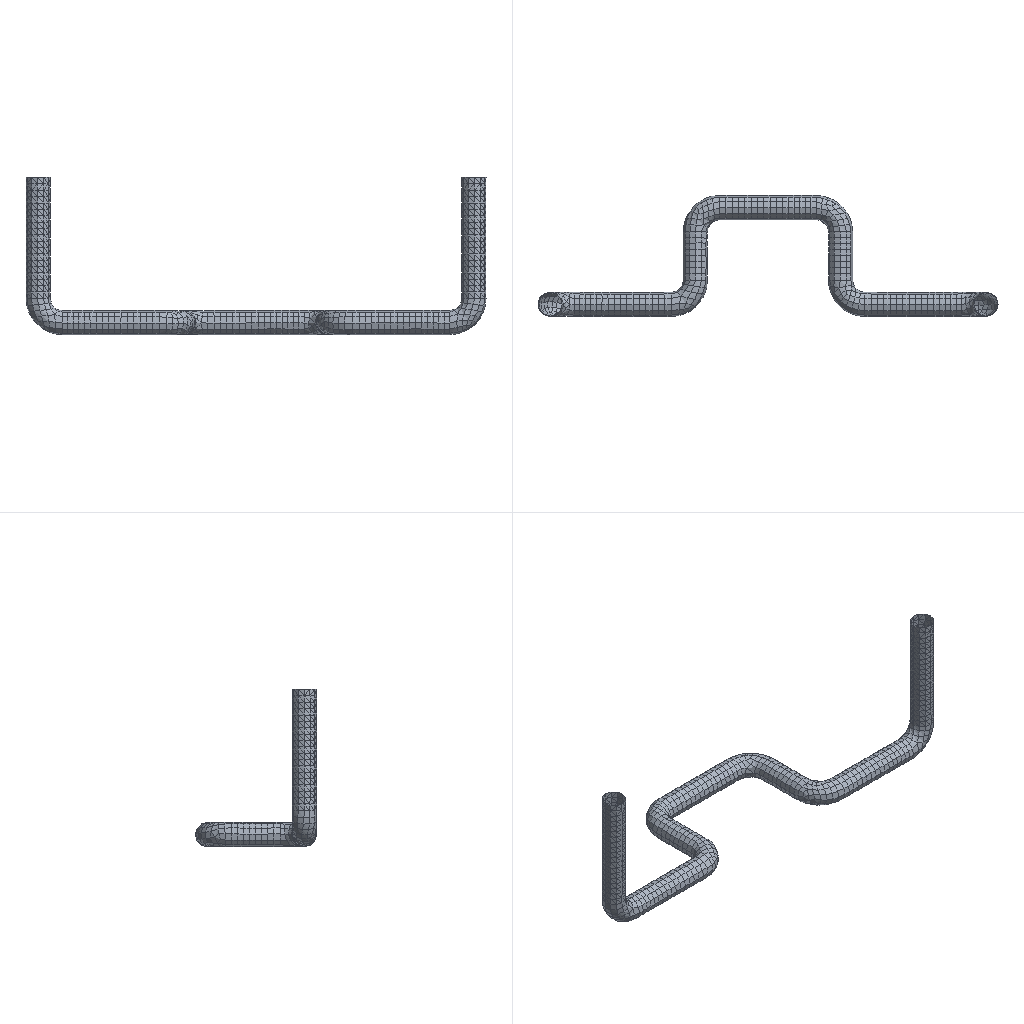Simulation study | ansys workbench
Set-up summary:
category,name,step,type,value,unit,region
solver,ansys_workbench
units,mm-N-s-tonne (MPa),,stated,"/units,MPA"
analysis,LS1,,transient
load_step,LS1,LS1,transient,time=1
mesh,nodes,,,1720
mesh,elements,,,3874
element_type,SHELL181,,,1709
element_type,SURF154,,,1709
element_type,CONTA174,,,456
material,Structural Steel,,E,200000,tonne s^-2 mm^-1
material,Structural Steel,,nu,0.3
material,Structural Steel,,density,7.85e-09,tonne mm^-3
material,Structural Steel,,conductivity,60.5,tonne mm s^-3 C^-1
material,Structural Steel,,specific_heat,4.34e+08,mm^2 s^-2 C^-1
material,Structural Steel,,cte,1.2e-05,C^-1
material,Structural Steel,,permeability,10000
material,Structural Steel,,resistivity,0.00017,ohm mm
load,ACEL,LS1,gravity (ACEL; gravity acts opposite),"9806.65 [dir=(0, -1, 0)]",,all
load,"Create Imported Load ""Imported Pressure""",LS1,pressure,1.094 [n=1709],,element list
bc,Constant Zero Displacement X,model,fixed,[dofs=UX],,_DISPZEROUX
bc,Constant Zero Displacement Z,model,fixed,[dofs=UZ],,_DISPZEROUZ
bc,"Create Spring Connection ""Longitudinal - Ground To Surface Body""",model,fixed,[dofs=ALL n=2],,node list
contact,contact 1,,bonded (always),element=CONTA174
contact,contact 2,,bonded (always),element=CONTA174
named_set,WALL,,node,1716
named_set,_DISPZEROUX,,node,1716
named_set,_DISPZEROUZ,,node,1716
named_set,ALLGROUNDEDSPRINGS,,node,2
Ansys APDL input file, long lists of numbers shortened:
/batch
/config,noeldb,1     ! force off writing results to database
*get,_wallstrt,active,,time,wall
! ANSYS input file written by Workbench version 2023 R1
! File used for geometry attach:
/title,E16sk--Transient (B5)
! ****** Begin Custom Load Command Snippet ******
/COM, ACT Extensions:
/COM,     LSDYNA, 2023.1
/COM,/COM,     ANSYSMotion, 2023.1
/COM,
! ****** End   Custom Load Command Snippet ******
*DIM,_wb_ProjectScratch_dir,string,248
_wb_ProjectScratch_dir(1) = ''
*DIM,_wb_SolverFiles_dir,string,248
_wb_SolverFiles_dir(1) = ''
*DIM,_wb_userfiles_dir,string,248
_wb_userfiles_dir(1) = ''
/com,--- Data in consistent NMM units. See Solving Units in the help system for more information.
/units,MPA
/nopr
/wb,file,start              !  signify a WB generated input file
/prep7
! Turn off shape checking because checks already performed inside WB mesher.
! See help system for more information.
SHPP,OFF,,NOWARN
/nolist
etcon,set             ! allow ANSYS to choose best KEYOP's for 180x elements, resets any applicable keyopt to MAPDL defaults
/com,*********** Nodes for the whole assembly ***********
nblock,3,,1887
(1i9,3e20.9e3)
        1    -1.250000000E+01     1.530808499E-15     1.500000000E+02
! (1715 more lines like these left out)
-1
/com,*********** Nodes for all Remote Points ***********
nblock,3
(1i9,3e20.9e3)
     1717     2.591630072E-16    -1.000000000E+02     8.750000317E+01
     1718     2.591630072E-16    -1.930224481E-16     8.750000317E+01
     1719     4.500000030E+02    -1.000000000E+02     8.750000317E+01
     1720     4.500000030E+02     2.875089333E-16     8.750000317E+01
-1
/wb,elem,start            !  set before creation of elements
/com,*********** Elements for Body 1 "Surface Body" ***********
et,1,181
keyo,1,1,0       ! bending and membrane stiffness
keyo,1,3,2
eblock,19,solid,,1709
(19i9)
        1        1        1        1        0        0        0        0        4        0     1011     1098     1065     1094     1094
! (1708 more lines like these left out)
-1
/wb,elem,end               !  done creating elements
/com,*********** Send User Defined Coordinate System(s) ***********
csys,0
toffst,273.15,  ! Temperature offset from absolute zero
/com,*********** Set Reference Temperature ***********
tref,22.
/wb,mat,start              !  starting to send materials
/com,*********** Send Materials ***********
Temperature = 'TEMP' ! Temperature
MP,DENS,1,7.85e-09,	! tonne mm^-3
MP,ALPX,1,1.2e-05,	! C^-1
MP,C,1,434000000,	! mm^2 s^-2 C^-1
MP,KXX,1,60.5,	! tonne mm s^-3 C^-1
MP,RSVX,1,0.00017,	! ohm mm
MP,EX,1,200000,	! tonne s^-2 mm^-1
MP,NUXY,1,0.3,
MP,MURX,1,10000,
/wb,mat,end                !  done sending materials
/com,*********** Send Sheet Properties ***********
sectype,1,shell
secdata,5.
secoff,mid
!************************* Model Summary ********************
!Surface Body,	Structural Steel,	matid,	1
!************************* End Model Summary ********************
! get the diagonal of the bounding box. Needed later for other things
*get,_xmin,node,,mnloc,x
*get,_ymin,node,,mnloc,y
*get,_zmin,node,,mnloc,z
*get,_xmax,node,,mxloc,x
*get,_ymax,node,,mxloc,y
*get,_zmax,node,,mxloc,z
_ASMDIAG=(_xmax-_xmin)*(_xmax-_xmin)+(_ymax-_ymin)*(_ymax-_ymin)+(_zmax-_zmin)*(_zmax-_zmin)
_ASMDIAG=SQRT(_ASMDIAG)
/wb,contact,start          !  starting to send contact
/wb,contact,end            !  done creating contacts
/com,*********** Send Named Selection as Node Component ***********
CMBLOCK,WALL    ,NODE,     1716
(8i10)
         1         2         3         4         5         6         7         8
! (214 more lines like these left out)
/golist
/wb,load,start             !  starting to send loads
/com,******* Constant Zero Displacement X *******
CMBLOCK,_DISPZEROUX,NODE,     1716
(8i10)
         1         2         3         4         5         6         7         8
! (214 more lines like these left out)
cmsel,s,_DISPZEROUX
d,all,ux,0
nsel,all
/com,******* Constant Zero Displacement Z *******
CMBLOCK,_DISPZEROUZ,NODE,     1716
(8i10)
         1         2         3         4         5         6         7         8
! (214 more lines like these left out)
cmsel,s,_DISPZEROUZ
d,all,uz,0
nsel,all
/com,*********** Create Remote Point "Internal Remote Point 2" ***********
! -------- Remote Point Used by "Longitudinal - Ground To Surface Body" --------
*set,tid,3
*set,cid,2
et,cid,174
et,tid,170
keyo,tid,2,1               ! Don't fix the pilot node
keyo,tid,4,111111
keyo,cid,12,5              ! Bonded Contact
keyo,cid,4,2               ! Rigid CERIG style load
keyo,cid,2,2               ! MPC style contact
eblock,10,,,228
(15i9)
     1716        2        2        2        0     1702     1502       12        1
! (227 more lines like these left out)
-1
*set,_npilot,1718
_npilot37=_npilot
type,tid
mat ,cid
real,cid
tshape,pilo
en,1944,_npilot
tshape
/com,*********** Create Remote Point "Internal Remote Point 4" ***********
! -------- Remote Point Used by "Longitudinal - Ground To Surface Body" --------
*set,tid,5
*set,cid,4
et,cid,174
et,tid,170
keyo,tid,2,1               ! Don't fix the pilot node
keyo,tid,4,111111
keyo,cid,12,5              ! Bonded Contact
keyo,cid,4,2               ! Rigid CERIG style load
keyo,cid,2,2               ! MPC style contact
eblock,10,,,228
(15i9)
     1945        4        4        4        0      172      174      356      367
! (227 more lines like these left out)
-1
*set,_npilot,1720
_npilot41=_npilot
type,tid
mat ,cid
real,cid
tshape,pilo
en,2173,_npilot
tshape
/com,*********** Create Spring Connection "Longitudinal - Ground To Surface Body" ***********
!
! Setup Spring Connection For Reference Set which is Grounded
d,1717,all
/com,            Real Constant Set For Above Spring Connection Is 6
*set,_sid,6
et,_sid,14            ! Combin14, Spring-Damper Element
mat,_sid
real,_sid
type,_sid
keyo,_sid,3,0           ! longitudinal  spring/damper
r,_sid,100000.,0.
en,1710,1717,1718
/com,*********** Create Spring Connection "Longitudinal - Ground To Surface Body" ***********
!
! Setup Spring Connection For Reference Set which is Grounded
d,1719,all
/com,            Real Constant Set For Above Spring Connection Is 7
*set,_sid,7
et,_sid,14            ! Combin14, Spring-Damper Element
mat,_sid
real,_sid
type,_sid
keyo,_sid,3,0           ! longitudinal  spring/damper
r,_sid,100000.,0.
en,1711,1719,1720
/COM,*** Create a component for all grounded springs ***
CMBLOCK,ALLGROUNDEDSPRINGS,NODE,        2
(8i10)
      1717      1719
/com,*********** Define Surface Elements for Imported Load "Imported Pressure" ***********
et,8,154
keyop,8,7,1				 ! Use original area so load is constant in large deformation
keyop,8,11,2               ! Use real and not projected area
eblock,10,,,1709
(15i9)
     2174        8        8        8        0      861      863     1031     1010
! (1708 more lines like these left out)
-1
esel,all
/gst,on,on
fini
*get,_numnode,node,0,count
*get,_numelem,elem,0,count
*get, _MAXELEMNUM, elem, 0, NUM, MAX
*get, _MAXNODENUM, node, 0, NUM, MAX
*get, _MAXELEMTYPE, etyp, 0, NUM, MAX
*get, _MAXREALCONST, rcon, 0, NUM, MAX
/go
/wb,load,end               !  done creating loads
/com,--- Number of total nodes = %_numnode%
/com,--- Number of contact elements = 456
/com,--- Number of spring elements = 0
/com,--- Number of bearing elements = 0
/com,--- Number of solid elements = 1709
/com,--- Number of condensed parts = 0
/com,--- Number of total elements = %_numelem%
*get,_wallbsol,active,,time,wall
/com,****************************************************************************
/com,*************************    SOLUTION       ********************************
/com,****************************************************************************
/solu
antype,4                   ! transient analysis
kbc,1                      ! stepped BC's
_thickRatio=  0     ! Ratio of thick parts in the model
eqsl,sparse,,,,,1
cntr,print,1               ! print out contact info and also make no initial contact an error
trnopt,full,,,,,hht        ! HHT time integration method
tintp, mosp			! Choose transient integration settings for moderate speed application
nldiag,cont,iter           ! print out contact info each equilibrium iteration
rescontrol,define,last,last,,dele	   ! Program Controlled
/com,****************************************************
/com,******************* SOLVE FOR LS 1 OF 1 ****************
acel,0.,9806.65,0.
/nopr
/com,*********** Create Imported Load "Imported Pressure" ***********
/nopr
sfe,2174,1,pres,0,1.035
sfe,2175,1,pres,0,1.032
sfe,2176,1,pres,0,1.039
sfe,2177,1,pres,0,1.04
! (1705 more lines like these left out)
/gopr
autots,off                 ! User turned off automatic time stepping
deltim,0.2,0.2,0.2
time,1.
timint,on                  ! Turn on time integration effects
outres,erase
outres,all,none
outres,nsol,all,
outres,rsol,all
outres,eangl,all
outres,etmp,all
outres,veng,all
outres,strs,all,
outres,epel,all,
outres,eppl,all,
outres,cont,all,
outres,v,all,
outres,a,all,
/nopr
esel,s,type,,6
esel,a,type,,7
cm,_elmisc,elem
esel,all
/gopr
outres,misc,all,_elmisc
! *********** WB SOLVE COMMAND ***********
! check interactive state
*get,ANSINTER_,active,,int
*if,ANSINTER_,ne,0,then
/eof
*endif
solve
/com *************** Write FE CONNECTORS *********
CEWRITE,file,ce,,INTE
/com,****************************************************
/com,*************** FINISHED SOLVE FOR LS 1 *************
*get,_wallasol,active,,time,wall
/nopr
*get,_numnode,node,0,count
*get,_numelem,elem,0,count
*get, _MAXELEMNUM, elem, 0, NUM, MAX
*get, _MAXNODENUM, node, 0, NUM, MAX,,,INTERNAL
*get, _MAXELEMTYPE, etyp, 0, NUM, MAX
*get, _MAXREALCONST, rcon, 0, NUM, MAX
*get,_NSOLTHREADS,active,0,ntfs
*get,_NSOLPROCESSES,active,0,npfs
/gopr
/post1
xmlo,ENCODING,ISO-8859-1
xmlo,parm
/xml,parm,xml
fini
/gopr
*get,_walldone,active,,time,wall
_preptime=(_wallbsol-_wallstrt)*3600
_solvtime=(_wallasol-_wallbsol)*3600
_posttime=(_walldone-_wallasol)*3600
_totaltim=(_walldone-_wallstrt)*3600
*get,_dlbratio,active,0,solu,dlbr
*get,_combtime,active,0,solu,comb
*get,_ssmode,active,0,solu,ssmm
*get,_ndofs,active,0,solu,ndof
/com,--- Total number of nodes = %_numnode%
/com,--- Total number of elements = %_numelem%
/com,--- Element load balance ratio = %_dlbratio%
/com,--- Time to combine distributed files = %_combtime%
/com,--- Sparse memory mode = %_ssmode%
/com,--- Number of DOF = %_ndofs%
/wb,file,end               ! done with WB generated input
Results summary:
result,analyses[0].index,,,1
result,analyses[0].system,,,SYS
result,analyses[0].deck,,,deck.dat
result,analyses[0].solve_status,,,completed
result,analyses[0].analysis_type,,,static
result,analyses[0].physics,,,mechanical
result,analyses[0].unit_system,,,"NMM: mm, ton, N, s, mV, mA, degC"
result,analyses[0].n_sets,,,5
result,analyses[0].load_steps[0].set,set=5,,5
result,analyses[0].load_steps[0].time_or_freq,set=5,,1
result,analyses[0].load_steps[0].max_displacement_magnitude,set=5,,0.001162
result,analyses[0].load_steps[0].max_von_mises_nodal,set=5,,3.208
result,analyses[0].load_steps[0].reaction_force_sum_xyz[1],set=5,,-9.355
result,analyses[0].load_steps[0].reaction_force_sum_xyz[2],set=5,,25.148
result,analyses[0].load_steps[0].reaction_force_sum_xyz[3],set=5,,-1066.98
result,geometry_export[0][0],,,1.step
result,geometry_export[0][1],,,ok
result,geometry_export[0][2],,,1
result,geometry_export[1][0],,,2.step
result,geometry_export[1][1],,,ok
result,geometry_export[1][2],,,1